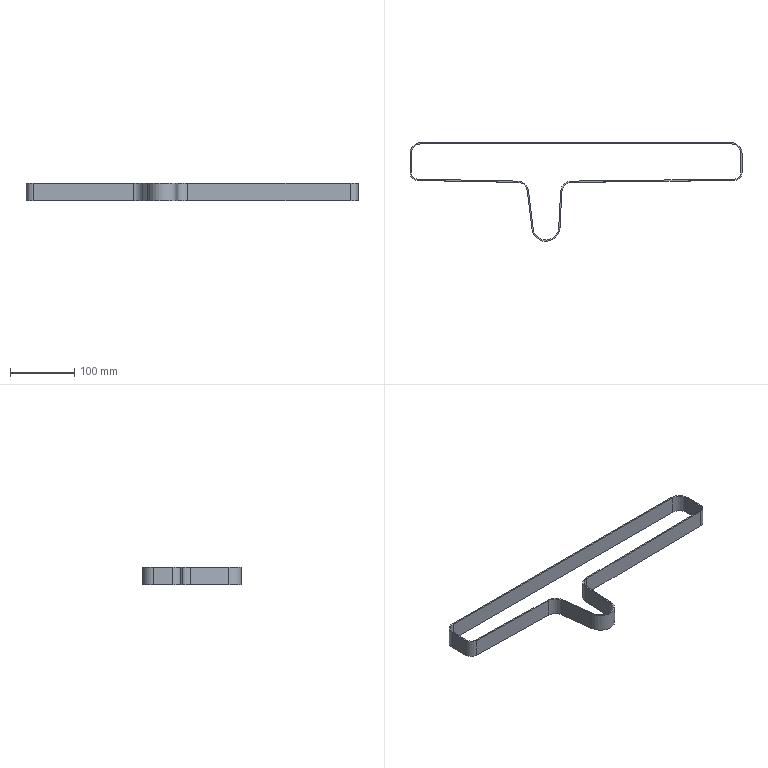Part | STEP file | Belt | 1 solid | 30 faces | box 518 x 154 x 28 mm | volume 70875 mm3 | plane 16 | cylinder 14 | commonest cylinder face diameters 30 x4 34 x4 20 x2 24 x2 40 x1 44 x1